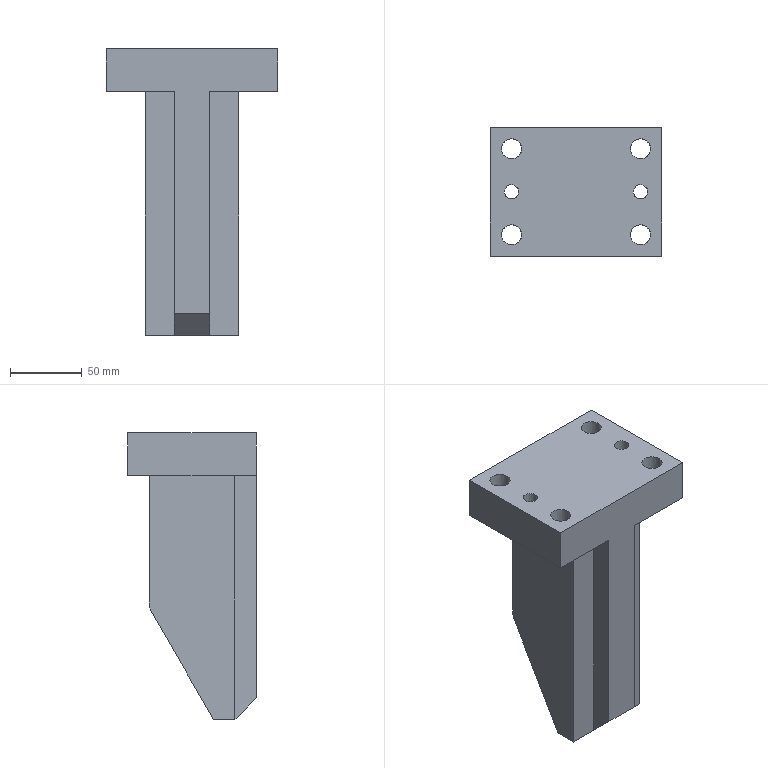Part | NX | features solid 2 | 1 solid | 35 faces | box 120 x 90 x 200 mm | volume 908928 mm3 | plane 22 | cylinder 13 | commonest cylinder face diameters 14 x4 20 x4 10 x2 11 x2 30 x1
STEP:
#1=CARTESIAN_POINT('',(32.5,540.,-38.));
#2=VERTEX_POINT('',#1);
#3=CARTESIAN_POINT('',(32.5,540.,-208.));
#4=VERTEX_POINT('',#3);
#5=CARTESIAN_POINT('',(32.5,540.,-18.));
#6=DIRECTION('',(0.,0.,-1.));
#7=VECTOR('',#6,1000.);
#8=LINE('',#5,#7);
#9=EDGE_CURVE('',#2,#4,#8,.T.);
#10=ORIENTED_EDGE('',*,*,#9,.F.);
#11=CARTESIAN_POINT('',(12.5,540.,-38.));
#12=VERTEX_POINT('',#11);
#13=CARTESIAN_POINT('',(12.5,540.,-38.));
#14=DIRECTION('',(-1.,0.,0.));
#15=VECTOR('',#14,1000.);
#16=LINE('',#13,#15);
#17=EDGE_CURVE('',#12,#2,#16,.F.);
#18=ORIENTED_EDGE('',*,*,#17,.F.);
#19=CARTESIAN_POINT('',(12.5,540.,-208.));
#20=VERTEX_POINT('',#19);
#21=CARTESIAN_POINT('',(12.5,540.,-18.));
#22=DIRECTION('',(0.,0.,-1.));
#23=VECTOR('',#22,1000.);
#24=LINE('',#21,#23);
#25=EDGE_CURVE('',#12,#20,#24,.T.);
#26=ORIENTED_EDGE('',*,*,#25,.T.);
#27=CARTESIAN_POINT('',(12.5,540.,-208.));
#28=DIRECTION('',(1.,0.,0.));
#29=VECTOR('',#28,1000.);
#30=LINE('',#27,#29);
#31=EDGE_CURVE('',#20,#4,#30,.T.);
#32=ORIENTED_EDGE('',*,*,#31,.T.);
#33=EDGE_LOOP('',(#10,#18,#26,#32));
#34=FACE_BOUND('',#33,.T.);
#35=CARTESIAN_POINT('',(12.5,540.,-18.));
#36=DIRECTION('',(0.,1.,0.));
#37=DIRECTION('',(0.,0.,1.));
#38=AXIS2_PLACEMENT_3D('',#35,#36,#37);
#39=PLANE('',#38);
#40=ADVANCED_FACE('',(#34),#39,.F.);
#41=CARTESIAN_POINT('',(32.5,555.,-208.));
#42=VERTEX_POINT('',#41);
#43=CARTESIAN_POINT('',(32.5,597.99,-133.538));
#44=VERTEX_POINT('',#43);
#45=CARTESIAN_POINT('',(32.5,600.,-130.058));
#46=DIRECTION('',(0.,0.5,0.866));
#47=VECTOR('',#46,1000.);
#48=LINE('',#45,#47);
#49=EDGE_CURVE('',#42,#44,#48,.T.);
#50=ORIENTED_EDGE('',*,*,#49,.T.);
#51=CARTESIAN_POINT('',(32.5,600.,-126.038));
#52=VERTEX_POINT('',#51);
#53=CARTESIAN_POINT('',(32.5,585.,-126.038));
#54=DIRECTION('',(-1.,0.,0.));
#55=DIRECTION('',(0.,-1.,0.));
#56=AXIS2_PLACEMENT_3D('',#53,#54,#55);
#57=CIRCLE('',#56,15.);
#58=EDGE_CURVE('',#44,#52,#57,.F.);
#59=ORIENTED_EDGE('',*,*,#58,.T.);
#60=CARTESIAN_POINT('',(32.5,600.,-38.));
#61=VERTEX_POINT('',#60);
#62=CARTESIAN_POINT('',(32.5,600.,-18.));
#63=DIRECTION('',(0.,0.,-1.));
#64=VECTOR('',#63,1000.);
#65=LINE('',#62,#64);
#66=EDGE_CURVE('',#61,#52,#65,.T.);
#67=ORIENTED_EDGE('',*,*,#66,.F.);
#68=CARTESIAN_POINT('',(32.5,615.,-38.));
#69=DIRECTION('',(0.,1.,0.));
#70=VECTOR('',#69,1000.);
#71=LINE('',#68,#70);
#72=EDGE_CURVE('',#2,#61,#71,.T.);
#73=ORIENTED_EDGE('',*,*,#72,.F.);
#74=ORIENTED_EDGE('',*,*,#9,.T.);
#75=CARTESIAN_POINT('',(32.5,540.,-208.));
#76=DIRECTION('',(0.,1.,0.));
#77=VECTOR('',#76,1000.);
#78=LINE('',#75,#77);
#79=EDGE_CURVE('',#4,#42,#78,.T.);
#80=ORIENTED_EDGE('',*,*,#79,.T.);
#81=EDGE_LOOP('',(#50,#59,#67,#73,#74,#80));
#82=FACE_BOUND('',#81,.T.);
#83=CARTESIAN_POINT('',(32.5,540.,-18.));
#84=DIRECTION('',(-1.,0.,0.));
#85=DIRECTION('',(0.,-1.,0.));
#86=AXIS2_PLACEMENT_3D('',#83,#84,#85);
#87=PLANE('',#86);
#88=ADVANCED_FACE('',(#82),#87,.F.);
#89=ORIENTED_EDGE('',*,*,#66,.T.);
#90=CARTESIAN_POINT('',(-32.5,600.,-126.038));
#91=VERTEX_POINT('',#90);
#92=CARTESIAN_POINT('',(-32.5,600.,-126.038));
#93=DIRECTION('',(-1.,0.,0.));
#94=VECTOR('',#93,1000.);
#95=LINE('',#92,#94);
#96=EDGE_CURVE('',#52,#91,#95,.T.);
#97=ORIENTED_EDGE('',*,*,#96,.T.);
#98=CARTESIAN_POINT('',(-32.5,600.,-38.));
#99=VERTEX_POINT('',#98);
#100=CARTESIAN_POINT('',(-32.5,600.,-18.));
#101=DIRECTION('',(0.,0.,-1.));
#102=VECTOR('',#101,1000.);
#103=LINE('',#100,#102);
#104=EDGE_CURVE('',#99,#91,#103,.T.);
#105=ORIENTED_EDGE('',*,*,#104,.F.);
#106=CARTESIAN_POINT('',(32.5,600.,-38.));
#107=DIRECTION('',(1.,0.,0.));
#108=VECTOR('',#107,1000.);
#109=LINE('',#106,#108);
#110=EDGE_CURVE('',#61,#99,#109,.F.);
#111=ORIENTED_EDGE('',*,*,#110,.F.);
#112=EDGE_LOOP('',(#89,#97,#105,#111));
#113=FACE_BOUND('',#112,.T.);
#114=CARTESIAN_POINT('',(32.5,600.,-18.));
#115=DIRECTION('',(0.,-1.,0.));
#116=DIRECTION('',(0.,0.,-1.));
#117=AXIS2_PLACEMENT_3D('',#114,#115,#116);
#118=PLANE('',#117);
#119=ADVANCED_FACE('',(#113),#118,.F.);
#120=ORIENTED_EDGE('',*,*,#104,.T.);
#121=CARTESIAN_POINT('',(-32.5,597.99,-133.538));
#122=VERTEX_POINT('',#121);
#123=CARTESIAN_POINT('',(-32.5,585.,-126.038));
#124=DIRECTION('',(1.,0.,0.));
#125=DIRECTION('',(0.,1.,0.));
#126=AXIS2_PLACEMENT_3D('',#123,#124,#125);
#127=CIRCLE('',#126,15.);
#128=EDGE_CURVE('',#91,#122,#127,.F.);
#129=ORIENTED_EDGE('',*,*,#128,.T.);
#130=CARTESIAN_POINT('',(-32.5,555.,-208.));
#131=VERTEX_POINT('',#130);
#132=CARTESIAN_POINT('',(-32.5,600.,-130.058));
#133=DIRECTION('',(0.,-0.5,-0.866));
#134=VECTOR('',#133,1000.);
#135=LINE('',#132,#134);
#136=EDGE_CURVE('',#122,#131,#135,.T.);
#137=ORIENTED_EDGE('',*,*,#136,.T.);
#138=CARTESIAN_POINT('',(-32.5,540.,-208.));
#139=VERTEX_POINT('',#138);
#140=CARTESIAN_POINT('',(-32.5,600.,-208.));
#141=DIRECTION('',(0.,-1.,0.));
#142=VECTOR('',#141,1000.);
#143=LINE('',#140,#142);
#144=EDGE_CURVE('',#131,#139,#143,.T.);
#145=ORIENTED_EDGE('',*,*,#144,.T.);
#146=CARTESIAN_POINT('',(-32.5,540.,-38.));
#147=VERTEX_POINT('',#146);
#148=CARTESIAN_POINT('',(-32.5,540.,-18.));
#149=DIRECTION('',(0.,0.,-1.));
#150=VECTOR('',#149,1000.);
#151=LINE('',#148,#150);
#152=EDGE_CURVE('',#147,#139,#151,.T.);
#153=ORIENTED_EDGE('',*,*,#152,.F.);
#154=CARTESIAN_POINT('',(-32.5,615.,-38.));
#155=DIRECTION('',(0.,-1.,0.));
#156=VECTOR('',#155,1000.);
#157=LINE('',#154,#156);
#158=EDGE_CURVE('',#99,#147,#157,.T.);
#159=ORIENTED_EDGE('',*,*,#158,.F.);
#160=EDGE_LOOP('',(#120,#129,#137,#145,#153,#159));
#161=FACE_BOUND('',#160,.T.);
#162=CARTESIAN_POINT('',(-32.5,600.,-18.));
#163=DIRECTION('',(1.,0.,0.));
#164=DIRECTION('',(0.,1.,0.));
#165=AXIS2_PLACEMENT_3D('',#162,#163,#164);
#166=PLANE('',#165);
#167=ADVANCED_FACE('',(#161),#166,.F.);
#168=CARTESIAN_POINT('',(-12.5,540.,-38.));
#169=VERTEX_POINT('',#168);
#170=CARTESIAN_POINT('',(-12.5,540.,-208.));
#171=VERTEX_POINT('',#170);
#172=CARTESIAN_POINT('',(-12.5,540.,-18.));
#173=DIRECTION('',(0.,0.,-1.));
#174=VECTOR('',#173,1000.);
#175=LINE('',#172,#174);
#176=EDGE_CURVE('',#169,#171,#175,.T.);
#177=ORIENTED_EDGE('',*,*,#176,.F.);
#178=CARTESIAN_POINT('',(12.5,540.,-38.));
#179=DIRECTION('',(-1.,0.,0.));
#180=VECTOR('',#179,1000.);
#181=LINE('',#178,#180);
#182=EDGE_CURVE('',#147,#169,#181,.F.);
#183=ORIENTED_EDGE('',*,*,#182,.F.);
#184=ORIENTED_EDGE('',*,*,#152,.T.);
#185=CARTESIAN_POINT('',(-32.5,540.,-208.));
#186=DIRECTION('',(1.,0.,0.));
#187=VECTOR('',#186,1000.);
#188=LINE('',#185,#187);
#189=EDGE_CURVE('',#139,#171,#188,.T.);
#190=ORIENTED_EDGE('',*,*,#189,.T.);
#191=EDGE_LOOP('',(#177,#183,#184,#190));
#192=FACE_BOUND('',#191,.T.);
#193=CARTESIAN_POINT('',(-32.5,540.,-18.));
#194=DIRECTION('',(0.,1.,0.));
#195=DIRECTION('',(0.,0.,1.));
#196=AXIS2_PLACEMENT_3D('',#193,#194,#195);
#197=PLANE('',#196);
#198=ADVANCED_FACE('',(#192),#197,.F.);
#199=CARTESIAN_POINT('',(-12.5,525.,-38.));
#200=VERTEX_POINT('',#199);
#201=CARTESIAN_POINT('',(-12.5,525.,-193.));
#202=VERTEX_POINT('',#201);
#203=CARTESIAN_POINT('',(-12.5,525.,-18.));
#204=DIRECTION('',(0.,0.,-1.));
#205=VECTOR('',#204,1000.);
#206=LINE('',#203,#205);
#207=EDGE_CURVE('',#200,#202,#206,.T.);
#208=ORIENTED_EDGE('',*,*,#207,.F.);
#209=CARTESIAN_POINT('',(-12.5,540.,-38.));
#210=DIRECTION('',(0.,1.,0.));
#211=VECTOR('',#210,1000.);
#212=LINE('',#209,#211);
#213=EDGE_CURVE('',#169,#200,#212,.F.);
#214=ORIENTED_EDGE('',*,*,#213,.F.);
#215=ORIENTED_EDGE('',*,*,#176,.T.);
#216=CARTESIAN_POINT('',(-12.5,525.,-193.));
#217=DIRECTION('',(0.,-0.7071,0.7071));
#218=VECTOR('',#217,1000.);
#219=LINE('',#216,#218);
#220=EDGE_CURVE('',#171,#202,#219,.T.);
#221=ORIENTED_EDGE('',*,*,#220,.T.);
#222=EDGE_LOOP('',(#208,#214,#215,#221));
#223=FACE_BOUND('',#222,.T.);
#224=CARTESIAN_POINT('',(-12.5,540.,-18.));
#225=DIRECTION('',(1.,0.,0.));
#226=DIRECTION('',(0.,1.,0.));
#227=AXIS2_PLACEMENT_3D('',#224,#225,#226);
#228=PLANE('',#227);
#229=ADVANCED_FACE('',(#223),#228,.F.);
#230=CARTESIAN_POINT('',(-60.,525.,-38.));
#231=VERTEX_POINT('',#230);
#232=CARTESIAN_POINT('',(-12.5,525.,-38.));
#233=DIRECTION('',(-1.,0.,0.));
#234=VECTOR('',#233,1000.);
#235=LINE('',#232,#234);
#236=EDGE_CURVE('',#200,#231,#235,.T.);
#237=ORIENTED_EDGE('',*,*,#236,.F.);
#238=ORIENTED_EDGE('',*,*,#207,.T.);
#239=CARTESIAN_POINT('',(12.5,525.,-193.));
#240=VERTEX_POINT('',#239);
#241=CARTESIAN_POINT('',(12.5,525.,-193.));
#242=DIRECTION('',(1.,0.,0.));
#243=VECTOR('',#242,1000.);
#244=LINE('',#241,#243);
#245=EDGE_CURVE('',#202,#240,#244,.T.);
#246=ORIENTED_EDGE('',*,*,#245,.T.);
#247=CARTESIAN_POINT('',(12.5,525.,-38.));
#248=VERTEX_POINT('',#247);
#249=CARTESIAN_POINT('',(12.5,525.,-18.));
#250=DIRECTION('',(0.,0.,-1.));
#251=VECTOR('',#250,1000.);
#252=LINE('',#249,#251);
#253=EDGE_CURVE('',#248,#240,#252,.T.);
#254=ORIENTED_EDGE('',*,*,#253,.F.);
#255=CARTESIAN_POINT('',(60.,525.,-38.));
#256=VERTEX_POINT('',#255);
#257=CARTESIAN_POINT('',(-12.5,525.,-38.));
#258=DIRECTION('',(-1.,0.,0.));
#259=VECTOR('',#258,1000.);
#260=LINE('',#257,#259);
#261=EDGE_CURVE('',#256,#248,#260,.T.);
#262=ORIENTED_EDGE('',*,*,#261,.F.);
#263=CARTESIAN_POINT('',(60.,525.,-8.));
#264=VERTEX_POINT('',#263);
#265=CARTESIAN_POINT('',(60.,525.,12.));
#266=DIRECTION('',(0.,0.,1.));
#267=VECTOR('',#266,1000.);
#268=LINE('',#265,#267);
#269=EDGE_CURVE('',#256,#264,#268,.T.);
#270=ORIENTED_EDGE('',*,*,#269,.T.);
#271=CARTESIAN_POINT('',(-60.,525.,-8.));
#272=VERTEX_POINT('',#271);
#273=CARTESIAN_POINT('',(60.,525.,-8.));
#274=DIRECTION('',(-1.,0.,0.));
#275=VECTOR('',#274,1000.);
#276=LINE('',#273,#275);
#277=EDGE_CURVE('',#264,#272,#276,.T.);
#278=ORIENTED_EDGE('',*,*,#277,.T.);
#279=CARTESIAN_POINT('',(-60.,525.,12.));
#280=DIRECTION('',(0.,0.,1.));
#281=VECTOR('',#280,1000.);
#282=LINE('',#279,#281);
#283=EDGE_CURVE('',#231,#272,#282,.T.);
#284=ORIENTED_EDGE('',*,*,#283,.F.);
#285=EDGE_LOOP('',(#237,#238,#246,#254,#262,#270,#278,#284));
#286=FACE_BOUND('',#285,.T.);
#287=CARTESIAN_POINT('',(-12.5,525.,-18.));
#288=DIRECTION('',(0.,1.,0.));
#289=DIRECTION('',(0.,0.,1.));
#290=AXIS2_PLACEMENT_3D('',#287,#288,#289);
#291=PLANE('',#290);
#292=ADVANCED_FACE('',(#286),#291,.F.);
#293=ORIENTED_EDGE('',*,*,#25,.F.);
#294=CARTESIAN_POINT('',(12.5,525.,-38.));
#295=DIRECTION('',(0.,-1.,0.));
#296=VECTOR('',#295,1000.);
#297=LINE('',#294,#296);
#298=EDGE_CURVE('',#248,#12,#297,.F.);
#299=ORIENTED_EDGE('',*,*,#298,.F.);
#300=ORIENTED_EDGE('',*,*,#253,.T.);
#301=CARTESIAN_POINT('',(12.5,525.,-193.));
#302=DIRECTION('',(0.,0.7071,-0.7071));
#303=VECTOR('',#302,1000.);
#304=LINE('',#301,#303);
#305=EDGE_CURVE('',#240,#20,#304,.T.);
#306=ORIENTED_EDGE('',*,*,#305,.T.);
#307=EDGE_LOOP('',(#293,#299,#300,#306));
#308=FACE_BOUND('',#307,.T.);
#309=CARTESIAN_POINT('',(12.5,525.,-18.));
#310=DIRECTION('',(-1.,0.,0.));
#311=DIRECTION('',(0.,-1.,0.));
#312=AXIS2_PLACEMENT_3D('',#309,#310,#311);
#313=PLANE('',#312);
#314=ADVANCED_FACE('',(#308),#313,.F.);
#315=ORIENTED_EDGE('',*,*,#144,.F.);
#316=CARTESIAN_POINT('',(32.5,555.,-208.));
#317=DIRECTION('',(1.,0.,0.));
#318=VECTOR('',#317,1000.);
#319=LINE('',#316,#318);
#320=EDGE_CURVE('',#131,#42,#319,.T.);
#321=ORIENTED_EDGE('',*,*,#320,.T.);
#322=ORIENTED_EDGE('',*,*,#79,.F.);
#323=ORIENTED_EDGE('',*,*,#31,.F.);
#324=CARTESIAN_POINT('',(-12.5,540.,-208.));
#325=DIRECTION('',(-1.,0.,0.));
#326=VECTOR('',#325,1000.);
#327=LINE('',#324,#326);
#328=EDGE_CURVE('',#20,#171,#327,.T.);
#329=ORIENTED_EDGE('',*,*,#328,.T.);
#330=ORIENTED_EDGE('',*,*,#189,.F.);
#331=EDGE_LOOP('',(#315,#321,#322,#323,#329,#330));
#332=FACE_BOUND('',#331,.T.);
#333=CARTESIAN_POINT('',(-12.5,540.,-208.));
#334=DIRECTION('',(0.,0.,-1.));
#335=DIRECTION('',(0.,1.,0.));
#336=AXIS2_PLACEMENT_3D('',#333,#334,#335);
#337=PLANE('',#336);
#338=ADVANCED_FACE('',(#332),#337,.T.);
#339=CARTESIAN_POINT('',(60.,615.,-38.));
#340=VERTEX_POINT('',#339);
#341=CARTESIAN_POINT('',(60.,615.,-38.));
#342=DIRECTION('',(0.,-1.,0.));
#343=VECTOR('',#342,1000.);
#344=LINE('',#341,#343);
#345=EDGE_CURVE('',#340,#256,#344,.T.);
#346=ORIENTED_EDGE('',*,*,#345,.F.);
#347=CARTESIAN_POINT('',(60.,615.,-8.));
#348=VERTEX_POINT('',#347);
#349=CARTESIAN_POINT('',(60.,615.,-8.));
#350=DIRECTION('',(0.,0.,1.));
#351=VECTOR('',#350,1000.);
#352=LINE('',#349,#351);
#353=EDGE_CURVE('',#340,#348,#352,.T.);
#354=ORIENTED_EDGE('',*,*,#353,.T.);
#355=CARTESIAN_POINT('',(60.,615.,-8.));
#356=DIRECTION('',(0.,-1.,0.));
#357=VECTOR('',#356,1000.);
#358=LINE('',#355,#357);
#359=EDGE_CURVE('',#348,#264,#358,.T.);
#360=ORIENTED_EDGE('',*,*,#359,.T.);
#361=ORIENTED_EDGE('',*,*,#269,.F.);
#362=EDGE_LOOP('',(#346,#354,#360,#361));
#363=FACE_BOUND('',#362,.T.);
#364=CARTESIAN_POINT('',(60.,615.,-38.));
#365=DIRECTION('',(1.,0.,0.));
#366=DIRECTION('',(0.,0.,1.));
#367=AXIS2_PLACEMENT_3D('',#364,#365,#366);
#368=PLANE('',#367);
#369=ADVANCED_FACE('',(#363),#368,.T.);
#370=CARTESIAN_POINT('',(-60.,615.,-38.));
#371=VERTEX_POINT('',#370);
#372=CARTESIAN_POINT('',(-60.,615.,-38.));
#373=DIRECTION('',(0.,-1.,0.));
#374=VECTOR('',#373,1000.);
#375=LINE('',#372,#374);
#376=EDGE_CURVE('',#371,#231,#375,.T.);
#377=ORIENTED_EDGE('',*,*,#376,.T.);
#378=ORIENTED_EDGE('',*,*,#283,.T.);
#379=CARTESIAN_POINT('',(-60.,615.,-8.));
#380=VERTEX_POINT('',#379);
#381=CARTESIAN_POINT('',(-60.,615.,-8.));
#382=DIRECTION('',(0.,-1.,0.));
#383=VECTOR('',#382,1000.);
#384=LINE('',#381,#383);
#385=EDGE_CURVE('',#380,#272,#384,.T.);
#386=ORIENTED_EDGE('',*,*,#385,.F.);
#387=CARTESIAN_POINT('',(-60.,615.,-8.));
#388=DIRECTION('',(0.,0.,1.));
#389=VECTOR('',#388,1000.);
#390=LINE('',#387,#389);
#391=EDGE_CURVE('',#371,#380,#390,.T.);
#392=ORIENTED_EDGE('',*,*,#391,.F.);
#393=EDGE_LOOP('',(#377,#378,#386,#392));
#394=FACE_BOUND('',#393,.T.);
#395=CARTESIAN_POINT('',(-60.,525.,-38.));
#396=DIRECTION('',(-1.,0.,0.));
#397=DIRECTION('',(0.,0.,-1.));
#398=AXIS2_PLACEMENT_3D('',#395,#396,#397);
#399=PLANE('',#398);
#400=ADVANCED_FACE('',(#394),#399,.T.);
#401=CARTESIAN_POINT('',(-50.5,570.,-38.));
#402=VERTEX_POINT('',#401);
#403=CARTESIAN_POINT('',(-45.,570.,-38.));
#404=DIRECTION('',(0.,0.,1.));
#405=DIRECTION('',(-1.,0.,0.));
#406=AXIS2_PLACEMENT_3D('',#403,#404,#405);
#407=CIRCLE('',#406,5.5);
#408=EDGE_CURVE('',#402,#402,#407,.T.);
#409=ORIENTED_EDGE('',*,*,#408,.T.);
#410=EDGE_LOOP('',(#409));
#411=FACE_BOUND('',#410,.T.);
#412=CARTESIAN_POINT('',(-55.,600.,-38.));
#413=VERTEX_POINT('',#412);
#414=CARTESIAN_POINT('',(-45.,600.,-38.));
#415=DIRECTION('',(0.,0.,1.));
#416=DIRECTION('',(-1.,0.,0.));
#417=AXIS2_PLACEMENT_3D('',#414,#415,#416);
#418=CIRCLE('',#417,10.);
#419=EDGE_CURVE('',#413,#413,#418,.T.);
#420=ORIENTED_EDGE('',*,*,#419,.T.);
#421=EDGE_LOOP('',(#420));
#422=FACE_BOUND('',#421,.T.);
#423=CARTESIAN_POINT('',(-55.,540.,-38.));
#424=VERTEX_POINT('',#423);
#425=CARTESIAN_POINT('',(-45.,540.,-38.));
#426=DIRECTION('',(0.,0.,1.));
#427=DIRECTION('',(-1.,0.,0.));
#428=AXIS2_PLACEMENT_3D('',#425,#426,#427);
#429=CIRCLE('',#428,10.);
#430=EDGE_CURVE('',#424,#424,#429,.T.);
#431=ORIENTED_EDGE('',*,*,#430,.T.);
#432=EDGE_LOOP('',(#431));
#433=FACE_BOUND('',#432,.T.);
#434=CARTESIAN_POINT('',(35.,600.,-38.));
#435=VERTEX_POINT('',#434);
#436=CARTESIAN_POINT('',(45.,600.,-38.));
#437=DIRECTION('',(0.,0.,1.));
#438=DIRECTION('',(-1.,0.,0.));
#439=AXIS2_PLACEMENT_3D('',#436,#437,#438);
#440=CIRCLE('',#439,10.);
#441=EDGE_CURVE('',#435,#435,#440,.T.);
#442=ORIENTED_EDGE('',*,*,#441,.T.);
#443=EDGE_LOOP('',(#442));
#444=FACE_BOUND('',#443,.T.);
#445=CARTESIAN_POINT('',(35.,540.,-38.));
#446=VERTEX_POINT('',#445);
#447=CARTESIAN_POINT('',(45.,540.,-38.));
#448=DIRECTION('',(0.,0.,1.));
#449=DIRECTION('',(-1.,0.,0.));
#450=AXIS2_PLACEMENT_3D('',#447,#448,#449);
#451=CIRCLE('',#450,10.);
#452=EDGE_CURVE('',#446,#446,#451,.T.);
#453=ORIENTED_EDGE('',*,*,#452,.T.);
#454=EDGE_LOOP('',(#453));
#455=FACE_BOUND('',#454,.T.);
#456=CARTESIAN_POINT('',(39.5,570.,-38.));
#457=VERTEX_POINT('',#456);
#458=CARTESIAN_POINT('',(45.,570.,-38.));
#459=DIRECTION('',(0.,0.,1.));
#460=DIRECTION('',(-1.,0.,0.));
#461=AXIS2_PLACEMENT_3D('',#458,#459,#460);
#462=CIRCLE('',#461,5.5);
#463=EDGE_CURVE('',#457,#457,#462,.T.);
#464=ORIENTED_EDGE('',*,*,#463,.T.);
#465=EDGE_LOOP('',(#464));
#466=FACE_BOUND('',#465,.T.);
#467=ORIENTED_EDGE('',*,*,#110,.T.);
#468=ORIENTED_EDGE('',*,*,#158,.T.);
#469=ORIENTED_EDGE('',*,*,#182,.T.);
#470=ORIENTED_EDGE('',*,*,#213,.T.);
#471=ORIENTED_EDGE('',*,*,#236,.T.);
#472=ORIENTED_EDGE('',*,*,#376,.F.);
#473=CARTESIAN_POINT('',(60.,615.,-38.));
#474=DIRECTION('',(-1.,0.,0.));
#475=VECTOR('',#474,1000.);
#476=LINE('',#473,#475);
#477=EDGE_CURVE('',#340,#371,#476,.T.);
#478=ORIENTED_EDGE('',*,*,#477,.F.);
#479=ORIENTED_EDGE('',*,*,#345,.T.);
#480=ORIENTED_EDGE('',*,*,#261,.T.);
#481=ORIENTED_EDGE('',*,*,#298,.T.);
#482=ORIENTED_EDGE('',*,*,#17,.T.);
#483=ORIENTED_EDGE('',*,*,#72,.T.);
#484=EDGE_LOOP('',(#467,#468,#469,#470,#471,#472,#478,#479,#480,#481,#482,#483));
#485=FACE_BOUND('',#484,.T.);
#486=CARTESIAN_POINT('',(-60.,615.,-38.));
#487=DIRECTION('',(0.,0.,-1.));
#488=DIRECTION('',(1.,0.,0.));
#489=AXIS2_PLACEMENT_3D('',#486,#487,#488);
#490=PLANE('',#489);
#491=ADVANCED_FACE('',(#411,#422,#433,#444,#455,#466,#485),#490,.T.);
#492=ORIENTED_EDGE('',*,*,#353,.F.);
#493=ORIENTED_EDGE('',*,*,#477,.T.);
#494=ORIENTED_EDGE('',*,*,#391,.T.);
#495=CARTESIAN_POINT('',(60.,615.,-8.));
#496=DIRECTION('',(-1.,0.,0.));
#497=VECTOR('',#496,1000.);
#498=LINE('',#495,#497);
#499=EDGE_CURVE('',#348,#380,#498,.T.);
#500=ORIENTED_EDGE('',*,*,#499,.F.);
#501=EDGE_LOOP('',(#492,#493,#494,#500));
#502=FACE_BOUND('',#501,.T.);
#503=CARTESIAN_POINT('',(-60.,615.,-38.));
#504=DIRECTION('',(0.,1.,0.));
#505=DIRECTION('',(0.,0.,-1.));
#506=AXIS2_PLACEMENT_3D('',#503,#504,#505);
#507=PLANE('',#506);
#508=ADVANCED_FACE('',(#502),#507,.T.);
#509=CARTESIAN_POINT('',(-45.,565.,-8.));
#510=VERTEX_POINT('',#509);
#511=CARTESIAN_POINT('',(-45.,570.,-8.));
#512=DIRECTION('',(0.,0.,1.));
#513=DIRECTION('',(0.,-1.,0.));
#514=AXIS2_PLACEMENT_3D('',#511,#512,#513);
#515=CIRCLE('',#514,5.);
#516=EDGE_CURVE('',#510,#510,#515,.T.);
#517=ORIENTED_EDGE('',*,*,#516,.F.);
#518=EDGE_LOOP('',(#517));
#519=FACE_BOUND('',#518,.T.);
#520=CARTESIAN_POINT('',(-45.,593.,-8.));
#521=VERTEX_POINT('',#520);
#522=CARTESIAN_POINT('',(-45.,600.,-8.));
#523=DIRECTION('',(0.,0.,1.));
#524=DIRECTION('',(0.,-1.,0.));
#525=AXIS2_PLACEMENT_3D('',#522,#523,#524);
#526=CIRCLE('',#525,7.);
#527=EDGE_CURVE('',#521,#521,#526,.T.);
#528=ORIENTED_EDGE('',*,*,#527,.F.);
#529=EDGE_LOOP('',(#528));
#530=FACE_BOUND('',#529,.T.);
#531=CARTESIAN_POINT('',(-45.,533.,-8.));
#532=VERTEX_POINT('',#531);
#533=CARTESIAN_POINT('',(-45.,540.,-8.));
#534=DIRECTION('',(0.,0.,1.));
#535=DIRECTION('',(0.,-1.,0.));
#536=AXIS2_PLACEMENT_3D('',#533,#534,#535);
#537=CIRCLE('',#536,7.);
#538=EDGE_CURVE('',#532,#532,#537,.T.);
#539=ORIENTED_EDGE('',*,*,#538,.F.);
#540=EDGE_LOOP('',(#539));
#541=FACE_BOUND('',#540,.T.);
#542=CARTESIAN_POINT('',(45.,593.,-8.));
#543=VERTEX_POINT('',#542);
#544=CARTESIAN_POINT('',(45.,600.,-8.));
#545=DIRECTION('',(0.,0.,1.));
#546=DIRECTION('',(0.,-1.,0.));
#547=AXIS2_PLACEMENT_3D('',#544,#545,#546);
#548=CIRCLE('',#547,7.);
#549=EDGE_CURVE('',#543,#543,#548,.T.);
#550=ORIENTED_EDGE('',*,*,#549,.F.);
#551=EDGE_LOOP('',(#550));
#552=FACE_BOUND('',#551,.T.);
#553=CARTESIAN_POINT('',(45.,533.,-8.));
#554=VERTEX_POINT('',#553);
#555=CARTESIAN_POINT('',(45.,540.,-8.));
#556=DIRECTION('',(0.,0.,1.));
#557=DIRECTION('',(0.,-1.,0.));
#558=AXIS2_PLACEMENT_3D('',#555,#556,#557);
#559=CIRCLE('',#558,7.);
#560=EDGE_CURVE('',#554,#554,#559,.T.);
#561=ORIENTED_EDGE('',*,*,#560,.F.);
#562=EDGE_LOOP('',(#561));
#563=FACE_BOUND('',#562,.T.);
#564=CARTESIAN_POINT('',(45.,565.,-8.));
#565=VERTEX_POINT('',#564);
#566=CARTESIAN_POINT('',(45.,570.,-8.));
#567=DIRECTION('',(0.,0.,1.));
#568=DIRECTION('',(0.,-1.,0.));
#569=AXIS2_PLACEMENT_3D('',#566,#567,#568);
#570=CIRCLE('',#569,5.);
#571=EDGE_CURVE('',#565,#565,#570,.T.);
#572=ORIENTED_EDGE('',*,*,#571,.F.);
#573=EDGE_LOOP('',(#572));
#574=FACE_BOUND('',#573,.T.);
#575=ORIENTED_EDGE('',*,*,#359,.F.);
#576=ORIENTED_EDGE('',*,*,#499,.T.);
#577=ORIENTED_EDGE('',*,*,#385,.T.);
#578=ORIENTED_EDGE('',*,*,#277,.F.);
#579=EDGE_LOOP('',(#575,#576,#577,#578));
#580=FACE_BOUND('',#579,.T.);
#581=CARTESIAN_POINT('',(60.,615.,-8.));
#582=DIRECTION('',(0.,0.,1.));
#583=DIRECTION('',(-1.,0.,0.));
#584=AXIS2_PLACEMENT_3D('',#581,#582,#583);
#585=PLANE('',#584);
#586=ADVANCED_FACE('',(#519,#530,#541,#552,#563,#574,#580),#585,.T.);
#587=ORIENTED_EDGE('',*,*,#571,.T.);
#588=EDGE_LOOP('',(#587));
#589=FACE_BOUND('',#588,.T.);
#590=CARTESIAN_POINT('',(40.,570.,-24.));
#591=VERTEX_POINT('',#590);
#592=CARTESIAN_POINT('',(45.,570.,-24.));
#593=DIRECTION('',(0.,0.,1.));
#594=DIRECTION('',(-1.,0.,0.));
#595=AXIS2_PLACEMENT_3D('',#592,#593,#594);
#596=CIRCLE('',#595,5.);
#597=EDGE_CURVE('',#591,#591,#596,.T.);
#598=ORIENTED_EDGE('',*,*,#597,.F.);
#599=EDGE_LOOP('',(#598));
#600=FACE_BOUND('',#599,.T.);
#601=CARTESIAN_POINT('',(45.,570.,494771.999));
#602=DIRECTION('',(0.,0.,1.));
#603=DIRECTION('',(-1.,0.,0.));
#604=AXIS2_PLACEMENT_3D('',#601,#602,#603);
#605=CYLINDRICAL_SURFACE('',#604,5.);
#606=ADVANCED_FACE('',(#589,#600),#605,.F.);
#607=ORIENTED_EDGE('',*,*,#597,.T.);
#608=EDGE_LOOP('',(#607));
#609=FACE_BOUND('',#608,.T.);
#610=CARTESIAN_POINT('',(39.5,570.,-24.));
#611=VERTEX_POINT('',#610);
#612=CARTESIAN_POINT('',(45.,570.,-24.));
#613=DIRECTION('',(0.,0.,1.));
#614=DIRECTION('',(-1.,0.,0.));
#615=AXIS2_PLACEMENT_3D('',#612,#613,#614);
#616=CIRCLE('',#615,5.5);
#617=EDGE_CURVE('',#611,#611,#616,.T.);
#618=ORIENTED_EDGE('',*,*,#617,.F.);
#619=EDGE_LOOP('',(#618));
#620=FACE_BOUND('',#619,.T.);
#621=CARTESIAN_POINT('',(45.,570.,-24.));
#622=DIRECTION('',(0.,0.,1.));
#623=DIRECTION('',(-1.,0.,0.));
#624=AXIS2_PLACEMENT_3D('',#621,#622,#623);
#625=PLANE('',#624);
#626=ADVANCED_FACE('',(#609,#620),#625,.F.);
#627=ORIENTED_EDGE('',*,*,#617,.T.);
#628=EDGE_LOOP('',(#627));
#629=FACE_BOUND('',#628,.T.);
#630=ORIENTED_EDGE('',*,*,#463,.F.);
#631=EDGE_LOOP('',(#630));
#632=FACE_BOUND('',#631,.T.);
#633=CARTESIAN_POINT('',(45.,570.,-38.));
#634=DIRECTION('',(0.,0.,1.));
#635=DIRECTION('',(-1.,0.,0.));
#636=AXIS2_PLACEMENT_3D('',#633,#634,#635);
#637=CYLINDRICAL_SURFACE('',#636,5.5);
#638=ADVANCED_FACE('',(#629,#632),#637,.F.);
#639=ORIENTED_EDGE('',*,*,#560,.T.);
#640=EDGE_LOOP('',(#639));
#641=FACE_BOUND('',#640,.T.);
#642=CARTESIAN_POINT('',(38.,540.,-36.));
#643=VERTEX_POINT('',#642);
#644=CARTESIAN_POINT('',(45.,540.,-36.));
#645=DIRECTION('',(0.,0.,1.));
#646=DIRECTION('',(-1.,0.,0.));
#647=AXIS2_PLACEMENT_3D('',#644,#645,#646);
#648=CIRCLE('',#647,7.);
#649=EDGE_CURVE('',#643,#643,#648,.T.);
#650=ORIENTED_EDGE('',*,*,#649,.F.);
#651=EDGE_LOOP('',(#650));
#652=FACE_BOUND('',#651,.T.);
#653=CARTESIAN_POINT('',(45.,540.,494771.999));
#654=DIRECTION('',(0.,0.,1.));
#655=DIRECTION('',(-1.,0.,0.));
#656=AXIS2_PLACEMENT_3D('',#653,#654,#655);
#657=CYLINDRICAL_SURFACE('',#656,7.);
#658=ADVANCED_FACE('',(#641,#652),#657,.F.);
#659=ORIENTED_EDGE('',*,*,#649,.T.);
#660=EDGE_LOOP('',(#659));
#661=FACE_BOUND('',#660,.T.);
#662=CARTESIAN_POINT('',(35.,540.,-36.));
#663=VERTEX_POINT('',#662);
#664=CARTESIAN_POINT('',(45.,540.,-36.));
#665=DIRECTION('',(0.,0.,1.));
#666=DIRECTION('',(-1.,0.,0.));
#667=AXIS2_PLACEMENT_3D('',#664,#665,#666);
#668=CIRCLE('',#667,10.);
#669=EDGE_CURVE('',#663,#663,#668,.T.);
#670=ORIENTED_EDGE('',*,*,#669,.F.);
#671=EDGE_LOOP('',(#670));
#672=FACE_BOUND('',#671,.T.);
#673=CARTESIAN_POINT('',(45.,540.,-36.));
#674=DIRECTION('',(0.,0.,1.));
#675=DIRECTION('',(-1.,0.,0.));
#676=AXIS2_PLACEMENT_3D('',#673,#674,#675);
#677=PLANE('',#676);
#678=ADVANCED_FACE('',(#661,#672),#677,.F.);
#679=ORIENTED_EDGE('',*,*,#669,.T.);
#680=EDGE_LOOP('',(#679));
#681=FACE_BOUND('',#680,.T.);
#682=ORIENTED_EDGE('',*,*,#452,.F.);
#683=EDGE_LOOP('',(#682));
#684=FACE_BOUND('',#683,.T.);
#685=CARTESIAN_POINT('',(45.,540.,-38.));
#686=DIRECTION('',(0.,0.,1.));
#687=DIRECTION('',(-1.,0.,0.));
#688=AXIS2_PLACEMENT_3D('',#685,#686,#687);
#689=CYLINDRICAL_SURFACE('',#688,10.);
#690=ADVANCED_FACE('',(#681,#684),#689,.F.);
#691=ORIENTED_EDGE('',*,*,#220,.F.);
#692=ORIENTED_EDGE('',*,*,#328,.F.);
#693=ORIENTED_EDGE('',*,*,#305,.F.);
#694=ORIENTED_EDGE('',*,*,#245,.F.);
#695=EDGE_LOOP('',(#691,#692,#693,#694));
#696=FACE_BOUND('',#695,.T.);
#697=CARTESIAN_POINT('',(-12.5,525.,-193.));
#698=DIRECTION('',(0.,-0.7071,-0.7071));
#699=DIRECTION('',(0.,0.7071,-0.7071));
#700=AXIS2_PLACEMENT_3D('',#697,#698,#699);
#701=PLANE('',#700);
#702=ADVANCED_FACE('',(#696),#701,.T.);
#703=ORIENTED_EDGE('',*,*,#549,.T.);
#704=EDGE_LOOP('',(#703));
#705=FACE_BOUND('',#704,.T.);
#706=CARTESIAN_POINT('',(38.,600.,-36.));
#707=VERTEX_POINT('',#706);
#708=CARTESIAN_POINT('',(45.,600.,-36.));
#709=DIRECTION('',(0.,0.,1.));
#710=DIRECTION('',(-1.,0.,0.));
#711=AXIS2_PLACEMENT_3D('',#708,#709,#710);
#712=CIRCLE('',#711,7.);
#713=EDGE_CURVE('',#707,#707,#712,.T.);
#714=ORIENTED_EDGE('',*,*,#713,.F.);
#715=EDGE_LOOP('',(#714));
#716=FACE_BOUND('',#715,.T.);
#717=CARTESIAN_POINT('',(45.,600.,494771.999));
#718=DIRECTION('',(0.,0.,1.));
#719=DIRECTION('',(-1.,0.,0.));
#720=AXIS2_PLACEMENT_3D('',#717,#718,#719);
#721=CYLINDRICAL_SURFACE('',#720,7.);
#722=ADVANCED_FACE('',(#705,#716),#721,.F.);
#723=ORIENTED_EDGE('',*,*,#713,.T.);
#724=EDGE_LOOP('',(#723));
#725=FACE_BOUND('',#724,.T.);
#726=CARTESIAN_POINT('',(35.,600.,-36.));
#727=VERTEX_POINT('',#726);
#728=CARTESIAN_POINT('',(45.,600.,-36.));
#729=DIRECTION('',(0.,0.,1.));
#730=DIRECTION('',(-1.,0.,0.));
#731=AXIS2_PLACEMENT_3D('',#728,#729,#730);
#732=CIRCLE('',#731,10.);
#733=EDGE_CURVE('',#727,#727,#732,.T.);
#734=ORIENTED_EDGE('',*,*,#733,.F.);
#735=EDGE_LOOP('',(#734));
#736=FACE_BOUND('',#735,.T.);
#737=CARTESIAN_POINT('',(45.,600.,-36.));
#738=DIRECTION('',(0.,0.,1.));
#739=DIRECTION('',(-1.,0.,0.));
#740=AXIS2_PLACEMENT_3D('',#737,#738,#739);
#741=PLANE('',#740);
#742=ADVANCED_FACE('',(#725,#736),#741,.F.);
#743=ORIENTED_EDGE('',*,*,#733,.T.);
#744=EDGE_LOOP('',(#743));
#745=FACE_BOUND('',#744,.T.);
#746=ORIENTED_EDGE('',*,*,#441,.F.);
#747=EDGE_LOOP('',(#746));
#748=FACE_BOUND('',#747,.T.);
#749=CARTESIAN_POINT('',(45.,600.,-38.));
#750=DIRECTION('',(0.,0.,1.));
#751=DIRECTION('',(-1.,0.,0.));
#752=AXIS2_PLACEMENT_3D('',#749,#750,#751);
#753=CYLINDRICAL_SURFACE('',#752,10.);
#754=ADVANCED_FACE('',(#745,#748),#753,.F.);
#755=ORIENTED_EDGE('',*,*,#538,.T.);
#756=EDGE_LOOP('',(#755));
#757=FACE_BOUND('',#756,.T.);
#758=CARTESIAN_POINT('',(-52.,540.,-36.));
#759=VERTEX_POINT('',#758);
#760=CARTESIAN_POINT('',(-45.,540.,-36.));
#761=DIRECTION('',(0.,0.,1.));
#762=DIRECTION('',(-1.,0.,0.));
#763=AXIS2_PLACEMENT_3D('',#760,#761,#762);
#764=CIRCLE('',#763,7.);
#765=EDGE_CURVE('',#759,#759,#764,.T.);
#766=ORIENTED_EDGE('',*,*,#765,.F.);
#767=EDGE_LOOP('',(#766));
#768=FACE_BOUND('',#767,.T.);
#769=CARTESIAN_POINT('',(-45.,540.,494771.999));
#770=DIRECTION('',(0.,0.,1.));
#771=DIRECTION('',(-1.,0.,0.));
#772=AXIS2_PLACEMENT_3D('',#769,#770,#771);
#773=CYLINDRICAL_SURFACE('',#772,7.);
#774=ADVANCED_FACE('',(#757,#768),#773,.F.);
#775=ORIENTED_EDGE('',*,*,#765,.T.);
#776=EDGE_LOOP('',(#775));
#777=FACE_BOUND('',#776,.T.);
#778=CARTESIAN_POINT('',(-55.,540.,-36.));
#779=VERTEX_POINT('',#778);
#780=CARTESIAN_POINT('',(-45.,540.,-36.));
#781=DIRECTION('',(0.,0.,1.));
#782=DIRECTION('',(-1.,0.,0.));
#783=AXIS2_PLACEMENT_3D('',#780,#781,#782);
#784=CIRCLE('',#783,10.);
#785=EDGE_CURVE('',#779,#779,#784,.T.);
#786=ORIENTED_EDGE('',*,*,#785,.F.);
#787=EDGE_LOOP('',(#786));
#788=FACE_BOUND('',#787,.T.);
#789=CARTESIAN_POINT('',(-45.,540.,-36.));
#790=DIRECTION('',(0.,0.,1.));
#791=DIRECTION('',(-1.,0.,0.));
#792=AXIS2_PLACEMENT_3D('',#789,#790,#791);
#793=PLANE('',#792);
#794=ADVANCED_FACE('',(#777,#788),#793,.F.);
#795=ORIENTED_EDGE('',*,*,#785,.T.);
#796=EDGE_LOOP('',(#795));
#797=FACE_BOUND('',#796,.T.);
#798=ORIENTED_EDGE('',*,*,#430,.F.);
#799=EDGE_LOOP('',(#798));
#800=FACE_BOUND('',#799,.T.);
#801=CARTESIAN_POINT('',(-45.,540.,-38.));
#802=DIRECTION('',(0.,0.,1.));
#803=DIRECTION('',(-1.,0.,0.));
#804=AXIS2_PLACEMENT_3D('',#801,#802,#803);
#805=CYLINDRICAL_SURFACE('',#804,10.);
#806=ADVANCED_FACE('',(#797,#800),#805,.F.);
#807=ORIENTED_EDGE('',*,*,#527,.T.);
#808=EDGE_LOOP('',(#807));
#809=FACE_BOUND('',#808,.T.);
#810=CARTESIAN_POINT('',(-52.,600.,-36.));
#811=VERTEX_POINT('',#810);
#812=CARTESIAN_POINT('',(-45.,600.,-36.));
#813=DIRECTION('',(0.,0.,1.));
#814=DIRECTION('',(-1.,0.,0.));
#815=AXIS2_PLACEMENT_3D('',#812,#813,#814);
#816=CIRCLE('',#815,7.);
#817=EDGE_CURVE('',#811,#811,#816,.T.);
#818=ORIENTED_EDGE('',*,*,#817,.F.);
#819=EDGE_LOOP('',(#818));
#820=FACE_BOUND('',#819,.T.);
#821=CARTESIAN_POINT('',(-45.,600.,494771.999));
#822=DIRECTION('',(0.,0.,1.));
#823=DIRECTION('',(-1.,0.,0.));
#824=AXIS2_PLACEMENT_3D('',#821,#822,#823);
#825=CYLINDRICAL_SURFACE('',#824,7.);
#826=ADVANCED_FACE('',(#809,#820),#825,.F.);
#827=ORIENTED_EDGE('',*,*,#817,.T.);
#828=EDGE_LOOP('',(#827));
#829=FACE_BOUND('',#828,.T.);
#830=CARTESIAN_POINT('',(-55.,600.,-36.));
#831=VERTEX_POINT('',#830);
#832=CARTESIAN_POINT('',(-45.,600.,-36.));
#833=DIRECTION('',(0.,0.,1.));
#834=DIRECTION('',(-1.,0.,0.));
#835=AXIS2_PLACEMENT_3D('',#832,#833,#834);
#836=CIRCLE('',#835,10.);
#837=EDGE_CURVE('',#831,#831,#836,.T.);
#838=ORIENTED_EDGE('',*,*,#837,.F.);
#839=EDGE_LOOP('',(#838));
#840=FACE_BOUND('',#839,.T.);
#841=CARTESIAN_POINT('',(-45.,600.,-36.));
#842=DIRECTION('',(0.,0.,1.));
#843=DIRECTION('',(-1.,0.,0.));
#844=AXIS2_PLACEMENT_3D('',#841,#842,#843);
#845=PLANE('',#844);
#846=ADVANCED_FACE('',(#829,#840),#845,.F.);
#847=ORIENTED_EDGE('',*,*,#837,.T.);
#848=EDGE_LOOP('',(#847));
#849=FACE_BOUND('',#848,.T.);
#850=ORIENTED_EDGE('',*,*,#419,.F.);
#851=EDGE_LOOP('',(#850));
#852=FACE_BOUND('',#851,.T.);
#853=CARTESIAN_POINT('',(-45.,600.,-38.));
#854=DIRECTION('',(0.,0.,1.));
#855=DIRECTION('',(-1.,0.,0.));
#856=AXIS2_PLACEMENT_3D('',#853,#854,#855);
#857=CYLINDRICAL_SURFACE('',#856,10.);
#858=ADVANCED_FACE('',(#849,#852),#857,.F.);
#859=ORIENTED_EDGE('',*,*,#516,.T.);
#860=EDGE_LOOP('',(#859));
#861=FACE_BOUND('',#860,.T.);
#862=CARTESIAN_POINT('',(-50.,570.,-24.));
#863=VERTEX_POINT('',#862);
#864=CARTESIAN_POINT('',(-45.,570.,-24.));
#865=DIRECTION('',(0.,0.,1.));
#866=DIRECTION('',(-1.,0.,0.));
#867=AXIS2_PLACEMENT_3D('',#864,#865,#866);
#868=CIRCLE('',#867,5.);
#869=EDGE_CURVE('',#863,#863,#868,.T.);
#870=ORIENTED_EDGE('',*,*,#869,.F.);
#871=EDGE_LOOP('',(#870));
#872=FACE_BOUND('',#871,.T.);
#873=CARTESIAN_POINT('',(-45.,570.,494771.999));
#874=DIRECTION('',(0.,0.,1.));
#875=DIRECTION('',(-1.,0.,0.));
#876=AXIS2_PLACEMENT_3D('',#873,#874,#875);
#877=CYLINDRICAL_SURFACE('',#876,5.);
#878=ADVANCED_FACE('',(#861,#872),#877,.F.);
#879=ORIENTED_EDGE('',*,*,#869,.T.);
#880=EDGE_LOOP('',(#879));
#881=FACE_BOUND('',#880,.T.);
#882=CARTESIAN_POINT('',(-50.5,570.,-24.));
#883=VERTEX_POINT('',#882);
#884=CARTESIAN_POINT('',(-45.,570.,-24.));
#885=DIRECTION('',(0.,0.,1.));
#886=DIRECTION('',(-1.,0.,0.));
#887=AXIS2_PLACEMENT_3D('',#884,#885,#886);
#888=CIRCLE('',#887,5.5);
#889=EDGE_CURVE('',#883,#883,#888,.T.);
#890=ORIENTED_EDGE('',*,*,#889,.F.);
#891=EDGE_LOOP('',(#890));
#892=FACE_BOUND('',#891,.T.);
#893=CARTESIAN_POINT('',(-45.,570.,-24.));
#894=DIRECTION('',(0.,0.,1.));
#895=DIRECTION('',(-1.,0.,0.));
#896=AXIS2_PLACEMENT_3D('',#893,#894,#895);
#897=PLANE('',#896);
#898=ADVANCED_FACE('',(#881,#892),#897,.F.);
#899=ORIENTED_EDGE('',*,*,#889,.T.);
#900=EDGE_LOOP('',(#899));
#901=FACE_BOUND('',#900,.T.);
#902=ORIENTED_EDGE('',*,*,#408,.F.);
#903=EDGE_LOOP('',(#902));
#904=FACE_BOUND('',#903,.T.);
#905=CARTESIAN_POINT('',(-45.,570.,-38.));
#906=DIRECTION('',(0.,0.,1.));
#907=DIRECTION('',(-1.,0.,0.));
#908=AXIS2_PLACEMENT_3D('',#905,#906,#907);
#909=CYLINDRICAL_SURFACE('',#908,5.5);
#910=ADVANCED_FACE('',(#901,#904),#909,.F.);
#911=ORIENTED_EDGE('',*,*,#136,.F.);
#912=CARTESIAN_POINT('',(32.5,597.99,-133.538));
#913=DIRECTION('',(-1.,0.,0.));
#914=VECTOR('',#913,1000.);
#915=LINE('',#912,#914);
#916=EDGE_CURVE('',#122,#44,#915,.F.);
#917=ORIENTED_EDGE('',*,*,#916,.T.);
#918=ORIENTED_EDGE('',*,*,#49,.F.);
#919=ORIENTED_EDGE('',*,*,#320,.F.);
#920=EDGE_LOOP('',(#911,#917,#918,#919));
#921=FACE_BOUND('',#920,.T.);
#922=CARTESIAN_POINT('',(32.5,600.,-130.058));
#923=DIRECTION('',(0.,0.866,-0.5));
#924=DIRECTION('',(0.,0.5,0.866));
#925=AXIS2_PLACEMENT_3D('',#922,#923,#924);
#926=PLANE('',#925);
#927=ADVANCED_FACE('',(#921),#926,.T.);
#928=ORIENTED_EDGE('',*,*,#58,.F.);
#929=ORIENTED_EDGE('',*,*,#916,.F.);
#930=ORIENTED_EDGE('',*,*,#128,.F.);
#931=ORIENTED_EDGE('',*,*,#96,.F.);
#932=EDGE_LOOP('',(#928,#929,#930,#931));
#933=FACE_BOUND('',#932,.T.);
#934=CARTESIAN_POINT('',(32.5,585.,-126.038));
#935=DIRECTION('',(1.,0.,0.));
#936=DIRECTION('',(0.,0.,1.));
#937=AXIS2_PLACEMENT_3D('',#934,#935,#936);
#938=CYLINDRICAL_SURFACE('',#937,15.);
#939=ADVANCED_FACE('',(#933),#938,.T.);
#940=CLOSED_SHELL('',(#40,#88,#119,#167,#198,#229,#292,#314,#338,#369,#400,#491,#508,#586,#606,#626,#638,#658,#678,#690,#702,#722,#742,#754,#774,#794,#806,#826,#846,#858,#878,#898,#910,#927,#939));
#941=MANIFOLD_SOLID_BREP('',#940);
#942=(LENGTH_UNIT()NAMED_UNIT(*)SI_UNIT(.MILLI.,.METRE.));
#943=UNCERTAINTY_MEASURE_WITH_UNIT(LENGTH_MEASURE(0.00001),#942,'','');
#944=(NAMED_UNIT(*)PLANE_ANGLE_UNIT()SI_UNIT($,.RADIAN.));
#945=(NAMED_UNIT(*)SI_UNIT($,.STERADIAN.)SOLID_ANGLE_UNIT());
#946=(GEOMETRIC_REPRESENTATION_CONTEXT(3)GLOBAL_UNCERTAINTY_ASSIGNED_CONTEXT((#943))GLOBAL_UNIT_ASSIGNED_CONTEXT((#942,#944,#945))REPRESENTATION_CONTEXT('',''));
#947=ADVANCED_BREP_SHAPE_REPRESENTATION('',(#941),#946);